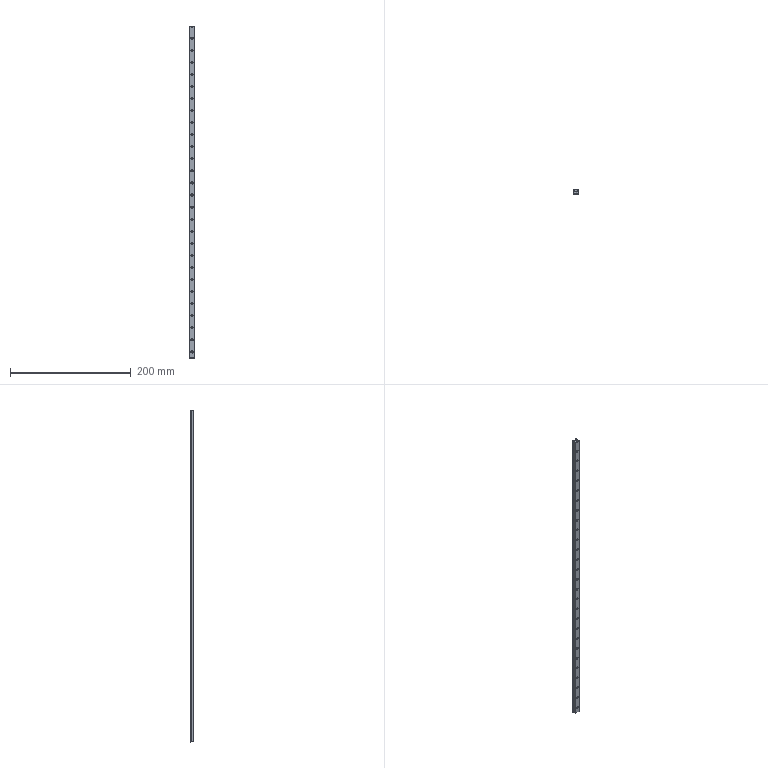Part | SolidWorks | features BaseBody 1 | 1 solid | 215 faces | box 9 x 6.5 x 550 mm | volume 27276 mm3 | cylinder 113 | cone 55 | plane 47 | commonest cylinder face diameters 3.5 x55 5.8 x55 0.8 x3